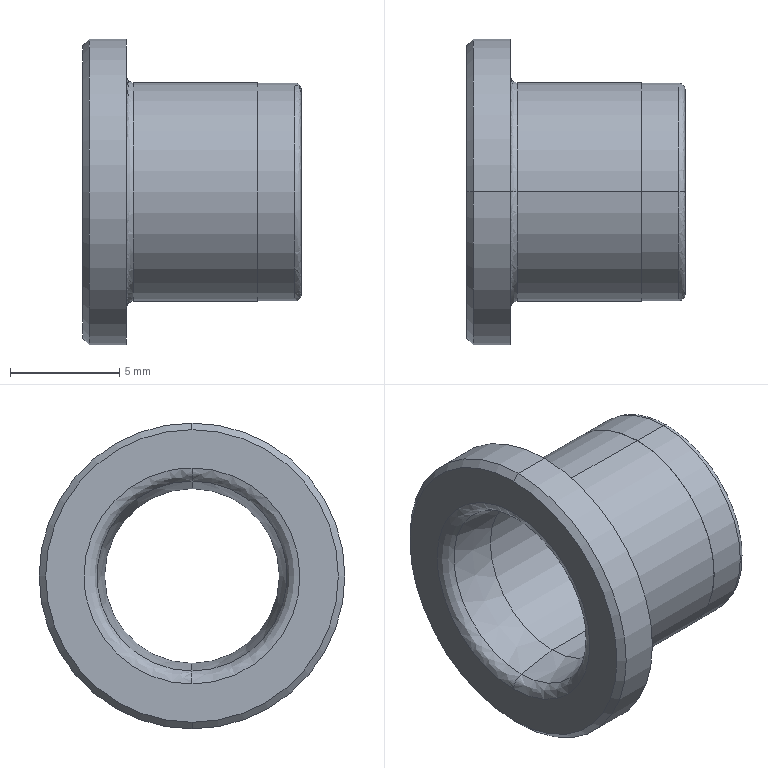Part | STEP file | 0217_016_MPFZU8-10 | 1 solid | 24 faces | box 10 x 14 x 14 mm | volume 412.979 mm3 | spline 8 | cylinder 8 | cone 4 | plane 4 | commonest cylinder face diameters 8 x2 9.98 x2 10 x2 14 x2